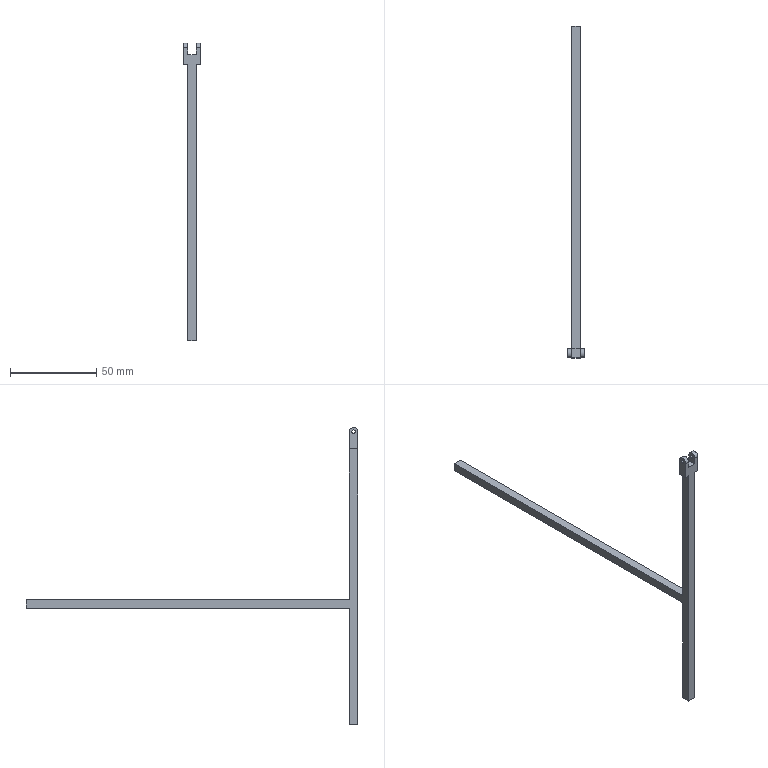Part | SolidWorks | features ICE 4, Extrusion 1 | 1 solid | 22 faces | box 10 x 192.5 x 172.5 mm | volume 9121 mm3 | plane 16 | cylinder 6 | commonest cylinder face diameters 2 x4 5 x2
STEP:
#1=CARTESIAN_POINT('',(2.5,-1.,170.));
#2=VERTEX_POINT('',#1);
#3=CARTESIAN_POINT('',(2.5,1.,170.));
#4=VERTEX_POINT('',#3);
#5=CARTESIAN_POINT('',(2.5,0.,170.));
#6=DIRECTION('',(1.,0.,0.));
#7=DIRECTION('',(0.,1.,0.));
#8=AXIS2_PLACEMENT_3D('',#5,#6,#7);
#9=CIRCLE('',#8,1.);
#10=EDGE_CURVE('',#2,#4,#9,.T.);
#11=ORIENTED_EDGE('',*,*,#10,.F.);
#12=CARTESIAN_POINT('',(5.,-1.,170.));
#13=VERTEX_POINT('',#12);
#14=CARTESIAN_POINT('',(-5.,-1.,170.));
#15=DIRECTION('',(1.,0.,0.));
#16=VECTOR('',#15,1000.);
#17=LINE('',#14,#16);
#18=EDGE_CURVE('',#2,#13,#17,.T.);
#19=ORIENTED_EDGE('',*,*,#18,.T.);
#20=CARTESIAN_POINT('',(5.,1.,170.));
#21=VERTEX_POINT('',#20);
#22=CARTESIAN_POINT('',(5.,0.,170.));
#23=DIRECTION('',(-1.,0.,0.));
#24=DIRECTION('',(0.,-1.,0.));
#25=AXIS2_PLACEMENT_3D('',#22,#23,#24);
#26=CIRCLE('',#25,1.);
#27=EDGE_CURVE('',#21,#13,#26,.T.);
#28=ORIENTED_EDGE('',*,*,#27,.F.);
#29=CARTESIAN_POINT('',(-5.,1.,170.));
#30=DIRECTION('',(1.,0.,0.));
#31=VECTOR('',#30,1000.);
#32=LINE('',#29,#31);
#33=EDGE_CURVE('',#4,#21,#32,.T.);
#34=ORIENTED_EDGE('',*,*,#33,.F.);
#35=EDGE_LOOP('',(#11,#19,#28,#34));
#36=FACE_OUTER_BOUND('',#35,.T.);
#37=CARTESIAN_POINT('',(-5.,0.,170.));
#38=DIRECTION('',(1.,0.,0.));
#39=DIRECTION('',(0.,1.,0.));
#40=AXIS2_PLACEMENT_3D('',#37,#38,#39);
#41=CYLINDRICAL_SURFACE('',#40,1.);
#42=ADVANCED_FACE('',(#36),#41,.F.);
#43=CARTESIAN_POINT('',(-5.,-1.,170.));
#44=VERTEX_POINT('',#43);
#45=CARTESIAN_POINT('',(-5.,1.,170.));
#46=VERTEX_POINT('',#45);
#47=CARTESIAN_POINT('',(-5.,0.,170.));
#48=DIRECTION('',(1.,0.,0.));
#49=DIRECTION('',(0.,1.,0.));
#50=AXIS2_PLACEMENT_3D('',#47,#48,#49);
#51=CIRCLE('',#50,1.);
#52=EDGE_CURVE('',#44,#46,#51,.T.);
#53=ORIENTED_EDGE('',*,*,#52,.F.);
#54=CARTESIAN_POINT('',(-2.5,-1.,170.));
#55=VERTEX_POINT('',#54);
#56=CARTESIAN_POINT('',(-5.,-1.,170.));
#57=DIRECTION('',(1.,0.,0.));
#58=VECTOR('',#57,1000.);
#59=LINE('',#56,#58);
#60=EDGE_CURVE('',#44,#55,#59,.T.);
#61=ORIENTED_EDGE('',*,*,#60,.T.);
#62=CARTESIAN_POINT('',(-2.5,1.,170.));
#63=VERTEX_POINT('',#62);
#64=CARTESIAN_POINT('',(-2.5,0.,170.));
#65=DIRECTION('',(-1.,0.,0.));
#66=DIRECTION('',(0.,-1.,0.));
#67=AXIS2_PLACEMENT_3D('',#64,#65,#66);
#68=CIRCLE('',#67,1.);
#69=EDGE_CURVE('',#63,#55,#68,.T.);
#70=ORIENTED_EDGE('',*,*,#69,.F.);
#71=CARTESIAN_POINT('',(-5.,1.,170.));
#72=DIRECTION('',(1.,0.,0.));
#73=VECTOR('',#72,1000.);
#74=LINE('',#71,#73);
#75=EDGE_CURVE('',#46,#63,#74,.T.);
#76=ORIENTED_EDGE('',*,*,#75,.F.);
#77=EDGE_LOOP('',(#53,#61,#70,#76));
#78=FACE_OUTER_BOUND('',#77,.T.);
#79=CARTESIAN_POINT('',(-5.,0.,170.));
#80=DIRECTION('',(1.,0.,0.));
#81=DIRECTION('',(0.,1.,0.));
#82=AXIS2_PLACEMENT_3D('',#79,#80,#81);
#83=CYLINDRICAL_SURFACE('',#82,1.);
#84=ADVANCED_FACE('',(#78),#83,.F.);
#85=CARTESIAN_POINT('',(2.5,2.5,67.5));
#86=VERTEX_POINT('',#85);
#87=CARTESIAN_POINT('',(-2.5,2.5,67.5));
#88=VERTEX_POINT('',#87);
#89=CARTESIAN_POINT('',(-2.5,2.5,67.5));
#90=DIRECTION('',(-1.,0.,0.));
#91=VECTOR('',#90,1000.);
#92=LINE('',#89,#91);
#93=EDGE_CURVE('',#86,#88,#92,.T.);
#94=ORIENTED_EDGE('',*,*,#93,.F.);
#95=CARTESIAN_POINT('',(2.5,2.5,0.));
#96=VERTEX_POINT('',#95);
#97=CARTESIAN_POINT('',(2.5,2.5,160.));
#98=DIRECTION('',(0.,0.,-1.));
#99=VECTOR('',#98,1000.);
#100=LINE('',#97,#99);
#101=EDGE_CURVE('',#86,#96,#100,.T.);
#102=ORIENTED_EDGE('',*,*,#101,.T.);
#103=CARTESIAN_POINT('',(-2.5,2.5,0.));
#104=VERTEX_POINT('',#103);
#105=CARTESIAN_POINT('',(-2.5,2.5,0.));
#106=DIRECTION('',(-1.,0.,0.));
#107=VECTOR('',#106,1000.);
#108=LINE('',#105,#107);
#109=EDGE_CURVE('',#96,#104,#108,.T.);
#110=ORIENTED_EDGE('',*,*,#109,.T.);
#111=CARTESIAN_POINT('',(-2.5,2.5,160.));
#112=DIRECTION('',(0.,0.,-1.));
#113=VECTOR('',#112,1000.);
#114=LINE('',#111,#113);
#115=EDGE_CURVE('',#88,#104,#114,.T.);
#116=ORIENTED_EDGE('',*,*,#115,.F.);
#117=EDGE_LOOP('',(#94,#102,#110,#116));
#118=FACE_OUTER_BOUND('',#117,.T.);
#119=CARTESIAN_POINT('',(-2.5,2.5,160.));
#120=DIRECTION('',(0.,-1.,0.));
#121=DIRECTION('',(0.,0.,-1.));
#122=AXIS2_PLACEMENT_3D('',#119,#120,#121);
#123=PLANE('',#122);
#124=ADVANCED_FACE('',(#118),#123,.F.);
#125=CARTESIAN_POINT('',(-2.5,2.5,72.5));
#126=VERTEX_POINT('',#125);
#127=CARTESIAN_POINT('',(2.5,2.5,72.5));
#128=VERTEX_POINT('',#127);
#129=CARTESIAN_POINT('',(-2.5,2.5,72.5));
#130=DIRECTION('',(1.,0.,0.));
#131=VECTOR('',#130,1000.);
#132=LINE('',#129,#131);
#133=EDGE_CURVE('',#126,#128,#132,.T.);
#134=ORIENTED_EDGE('',*,*,#133,.F.);
#135=CARTESIAN_POINT('',(-2.5,2.5,160.));
#136=VERTEX_POINT('',#135);
#137=CARTESIAN_POINT('',(-2.5,2.5,160.));
#138=DIRECTION('',(0.,0.,-1.));
#139=VECTOR('',#138,1000.);
#140=LINE('',#137,#139);
#141=EDGE_CURVE('',#136,#126,#140,.T.);
#142=ORIENTED_EDGE('',*,*,#141,.F.);
#143=CARTESIAN_POINT('',(-5.,2.5,160.));
#144=VERTEX_POINT('',#143);
#145=CARTESIAN_POINT('',(-5.,2.5,160.));
#146=DIRECTION('',(-1.,0.,0.));
#147=VECTOR('',#146,1000.);
#148=LINE('',#145,#147);
#149=EDGE_CURVE('',#136,#144,#148,.T.);
#150=ORIENTED_EDGE('',*,*,#149,.T.);
#151=CARTESIAN_POINT('',(-5.,2.5,170.));
#152=VERTEX_POINT('',#151);
#153=CARTESIAN_POINT('',(-5.,2.5,178.));
#154=DIRECTION('',(0.,0.,-1.));
#155=VECTOR('',#154,1000.);
#156=LINE('',#153,#155);
#157=EDGE_CURVE('',#152,#144,#156,.T.);
#158=ORIENTED_EDGE('',*,*,#157,.F.);
#159=CARTESIAN_POINT('',(-2.5,2.5,170.));
#160=VERTEX_POINT('',#159);
#161=CARTESIAN_POINT('',(-5.,2.5,170.));
#162=DIRECTION('',(1.,0.,0.));
#163=VECTOR('',#162,1000.);
#164=LINE('',#161,#163);
#165=EDGE_CURVE('',#152,#160,#164,.T.);
#166=ORIENTED_EDGE('',*,*,#165,.T.);
#167=CARTESIAN_POINT('',(-2.5,2.5,166.));
#168=VERTEX_POINT('',#167);
#169=CARTESIAN_POINT('',(-2.5,2.5,160.));
#170=DIRECTION('',(0.,0.,-1.));
#171=VECTOR('',#170,1000.);
#172=LINE('',#169,#171);
#173=EDGE_CURVE('',#160,#168,#172,.T.);
#174=ORIENTED_EDGE('',*,*,#173,.T.);
#175=CARTESIAN_POINT('',(2.5,2.5,166.));
#176=VERTEX_POINT('',#175);
#177=CARTESIAN_POINT('',(-2.5,2.5,166.));
#178=DIRECTION('',(-1.,0.,0.));
#179=VECTOR('',#178,1000.);
#180=LINE('',#177,#179);
#181=EDGE_CURVE('',#176,#168,#180,.T.);
#182=ORIENTED_EDGE('',*,*,#181,.F.);
#183=CARTESIAN_POINT('',(2.5,2.5,170.));
#184=VERTEX_POINT('',#183);
#185=CARTESIAN_POINT('',(2.5,2.5,160.));
#186=DIRECTION('',(0.,0.,1.));
#187=VECTOR('',#186,1000.);
#188=LINE('',#185,#187);
#189=EDGE_CURVE('',#176,#184,#188,.T.);
#190=ORIENTED_EDGE('',*,*,#189,.T.);
#191=CARTESIAN_POINT('',(5.,2.5,170.));
#192=VERTEX_POINT('',#191);
#193=CARTESIAN_POINT('',(-5.,2.5,170.));
#194=DIRECTION('',(1.,0.,0.));
#195=VECTOR('',#194,1000.);
#196=LINE('',#193,#195);
#197=EDGE_CURVE('',#184,#192,#196,.T.);
#198=ORIENTED_EDGE('',*,*,#197,.T.);
#199=CARTESIAN_POINT('',(5.,2.5,160.));
#200=VERTEX_POINT('',#199);
#201=CARTESIAN_POINT('',(5.,2.5,178.));
#202=DIRECTION('',(0.,0.,-1.));
#203=VECTOR('',#202,1000.);
#204=LINE('',#201,#203);
#205=EDGE_CURVE('',#192,#200,#204,.T.);
#206=ORIENTED_EDGE('',*,*,#205,.T.);
#207=CARTESIAN_POINT('',(2.5,2.5,160.));
#208=VERTEX_POINT('',#207);
#209=CARTESIAN_POINT('',(-5.,2.5,160.));
#210=DIRECTION('',(-1.,0.,0.));
#211=VECTOR('',#210,1000.);
#212=LINE('',#209,#211);
#213=EDGE_CURVE('',#200,#208,#212,.T.);
#214=ORIENTED_EDGE('',*,*,#213,.T.);
#215=CARTESIAN_POINT('',(2.5,2.5,160.));
#216=DIRECTION('',(0.,0.,-1.));
#217=VECTOR('',#216,1000.);
#218=LINE('',#215,#217);
#219=EDGE_CURVE('',#208,#128,#218,.T.);
#220=ORIENTED_EDGE('',*,*,#219,.T.);
#221=EDGE_LOOP('',(#134,#142,#150,#158,#166,#174,#182,#190,#198,#206,#214,#220));
#222=FACE_OUTER_BOUND('',#221,.T.);
#223=CARTESIAN_POINT('',(-2.5,2.5,160.));
#224=DIRECTION('',(0.,-1.,0.));
#225=DIRECTION('',(0.,0.,-1.));
#226=AXIS2_PLACEMENT_3D('',#223,#224,#225);
#227=PLANE('',#226);
#228=ADVANCED_FACE('',(#222),#227,.F.);
#229=ORIENTED_EDGE('',*,*,#101,.F.);
#230=CARTESIAN_POINT('',(2.5,190.,67.5));
#231=VERTEX_POINT('',#230);
#232=CARTESIAN_POINT('',(2.5,190.,67.5));
#233=DIRECTION('',(0.,-1.,0.));
#234=VECTOR('',#233,1000.);
#235=LINE('',#232,#234);
#236=EDGE_CURVE('',#231,#86,#235,.T.);
#237=ORIENTED_EDGE('',*,*,#236,.F.);
#238=CARTESIAN_POINT('',(2.5,190.,72.5));
#239=VERTEX_POINT('',#238);
#240=CARTESIAN_POINT('',(2.5,190.,67.5));
#241=DIRECTION('',(0.,0.,-1.));
#242=VECTOR('',#241,1000.);
#243=LINE('',#240,#242);
#244=EDGE_CURVE('',#239,#231,#243,.T.);
#245=ORIENTED_EDGE('',*,*,#244,.F.);
#246=CARTESIAN_POINT('',(2.5,190.,72.5));
#247=DIRECTION('',(0.,-1.,0.));
#248=VECTOR('',#247,1000.);
#249=LINE('',#246,#248);
#250=EDGE_CURVE('',#239,#128,#249,.T.);
#251=ORIENTED_EDGE('',*,*,#250,.T.);
#252=ORIENTED_EDGE('',*,*,#219,.F.);
#253=CARTESIAN_POINT('',(2.5,-2.5,160.));
#254=VERTEX_POINT('',#253);
#255=CARTESIAN_POINT('',(2.5,2.5,160.));
#256=DIRECTION('',(0.,1.,0.));
#257=VECTOR('',#256,1000.);
#258=LINE('',#255,#257);
#259=EDGE_CURVE('',#254,#208,#258,.T.);
#260=ORIENTED_EDGE('',*,*,#259,.F.);
#261=CARTESIAN_POINT('',(2.5,-2.5,0.));
#262=VERTEX_POINT('',#261);
#263=CARTESIAN_POINT('',(2.5,-2.5,160.));
#264=DIRECTION('',(0.,0.,-1.));
#265=VECTOR('',#264,1000.);
#266=LINE('',#263,#265);
#267=EDGE_CURVE('',#254,#262,#266,.T.);
#268=ORIENTED_EDGE('',*,*,#267,.T.);
#269=CARTESIAN_POINT('',(2.5,2.5,0.));
#270=DIRECTION('',(0.,1.,0.));
#271=VECTOR('',#270,1000.);
#272=LINE('',#269,#271);
#273=EDGE_CURVE('',#262,#96,#272,.T.);
#274=ORIENTED_EDGE('',*,*,#273,.T.);
#275=EDGE_LOOP('',(#229,#237,#245,#251,#252,#260,#268,#274));
#276=FACE_OUTER_BOUND('',#275,.T.);
#277=CARTESIAN_POINT('',(2.5,2.5,160.));
#278=DIRECTION('',(-1.,0.,0.));
#279=DIRECTION('',(0.,-1.,0.));
#280=AXIS2_PLACEMENT_3D('',#277,#278,#279);
#281=PLANE('',#280);
#282=ADVANCED_FACE('',(#276),#281,.F.);
#283=ORIENTED_EDGE('',*,*,#141,.T.);
#284=CARTESIAN_POINT('',(-2.5,190.,72.5));
#285=VERTEX_POINT('',#284);
#286=CARTESIAN_POINT('',(-2.5,190.,72.5));
#287=DIRECTION('',(0.,-1.,0.));
#288=VECTOR('',#287,1000.);
#289=LINE('',#286,#288);
#290=EDGE_CURVE('',#285,#126,#289,.T.);
#291=ORIENTED_EDGE('',*,*,#290,.F.);
#292=CARTESIAN_POINT('',(-2.5,190.,67.5));
#293=VERTEX_POINT('',#292);
#294=CARTESIAN_POINT('',(-2.5,190.,67.5));
#295=DIRECTION('',(0.,0.,1.));
#296=VECTOR('',#295,1000.);
#297=LINE('',#294,#296);
#298=EDGE_CURVE('',#293,#285,#297,.T.);
#299=ORIENTED_EDGE('',*,*,#298,.F.);
#300=CARTESIAN_POINT('',(-2.5,190.,67.5));
#301=DIRECTION('',(0.,-1.,0.));
#302=VECTOR('',#301,1000.);
#303=LINE('',#300,#302);
#304=EDGE_CURVE('',#293,#88,#303,.T.);
#305=ORIENTED_EDGE('',*,*,#304,.T.);
#306=ORIENTED_EDGE('',*,*,#115,.T.);
#307=CARTESIAN_POINT('',(-2.5,-2.5,0.));
#308=VERTEX_POINT('',#307);
#309=CARTESIAN_POINT('',(-2.5,2.5,0.));
#310=DIRECTION('',(0.,-1.,0.));
#311=VECTOR('',#310,1000.);
#312=LINE('',#309,#311);
#313=EDGE_CURVE('',#104,#308,#312,.T.);
#314=ORIENTED_EDGE('',*,*,#313,.T.);
#315=CARTESIAN_POINT('',(-2.5,-2.5,160.));
#316=VERTEX_POINT('',#315);
#317=CARTESIAN_POINT('',(-2.5,-2.5,160.));
#318=DIRECTION('',(0.,0.,-1.));
#319=VECTOR('',#318,1000.);
#320=LINE('',#317,#319);
#321=EDGE_CURVE('',#316,#308,#320,.T.);
#322=ORIENTED_EDGE('',*,*,#321,.F.);
#323=CARTESIAN_POINT('',(-2.5,2.5,160.));
#324=DIRECTION('',(0.,-1.,0.));
#325=VECTOR('',#324,1000.);
#326=LINE('',#323,#325);
#327=EDGE_CURVE('',#136,#316,#326,.T.);
#328=ORIENTED_EDGE('',*,*,#327,.F.);
#329=EDGE_LOOP('',(#283,#291,#299,#305,#306,#314,#322,#328));
#330=FACE_OUTER_BOUND('',#329,.T.);
#331=CARTESIAN_POINT('',(-2.5,2.5,160.));
#332=DIRECTION('',(1.,0.,0.));
#333=DIRECTION('',(0.,1.,0.));
#334=AXIS2_PLACEMENT_3D('',#331,#332,#333);
#335=PLANE('',#334);
#336=ADVANCED_FACE('',(#330),#335,.F.);
#337=CARTESIAN_POINT('',(5.,-2.5,170.));
#338=VERTEX_POINT('',#337);
#339=CARTESIAN_POINT('',(5.,-2.5,160.));
#340=VERTEX_POINT('',#339);
#341=CARTESIAN_POINT('',(5.,-2.5,178.));
#342=DIRECTION('',(0.,0.,-1.));
#343=VECTOR('',#342,1000.);
#344=LINE('',#341,#343);
#345=EDGE_CURVE('',#338,#340,#344,.T.);
#346=ORIENTED_EDGE('',*,*,#345,.F.);
#347=CARTESIAN_POINT('',(2.5,-2.5,170.));
#348=VERTEX_POINT('',#347);
#349=CARTESIAN_POINT('',(-5.,-2.5,170.));
#350=DIRECTION('',(1.,0.,0.));
#351=VECTOR('',#350,1000.);
#352=LINE('',#349,#351);
#353=EDGE_CURVE('',#348,#338,#352,.T.);
#354=ORIENTED_EDGE('',*,*,#353,.F.);
#355=CARTESIAN_POINT('',(2.5,-2.5,166.));
#356=VERTEX_POINT('',#355);
#357=CARTESIAN_POINT('',(2.5,-2.5,160.));
#358=DIRECTION('',(0.,0.,-1.));
#359=VECTOR('',#358,1000.);
#360=LINE('',#357,#359);
#361=EDGE_CURVE('',#348,#356,#360,.T.);
#362=ORIENTED_EDGE('',*,*,#361,.T.);
#363=CARTESIAN_POINT('',(-2.5,-2.5,166.));
#364=VERTEX_POINT('',#363);
#365=CARTESIAN_POINT('',(-2.5,-2.5,166.));
#366=DIRECTION('',(1.,0.,0.));
#367=VECTOR('',#366,1000.);
#368=LINE('',#365,#367);
#369=EDGE_CURVE('',#364,#356,#368,.T.);
#370=ORIENTED_EDGE('',*,*,#369,.F.);
#371=CARTESIAN_POINT('',(-2.5,-2.5,170.));
#372=VERTEX_POINT('',#371);
#373=CARTESIAN_POINT('',(-2.5,-2.5,160.));
#374=DIRECTION('',(0.,0.,1.));
#375=VECTOR('',#374,1000.);
#376=LINE('',#373,#375);
#377=EDGE_CURVE('',#364,#372,#376,.T.);
#378=ORIENTED_EDGE('',*,*,#377,.T.);
#379=CARTESIAN_POINT('',(-5.,-2.5,170.));
#380=VERTEX_POINT('',#379);
#381=CARTESIAN_POINT('',(-5.,-2.5,170.));
#382=DIRECTION('',(1.,0.,0.));
#383=VECTOR('',#382,1000.);
#384=LINE('',#381,#383);
#385=EDGE_CURVE('',#380,#372,#384,.T.);
#386=ORIENTED_EDGE('',*,*,#385,.F.);
#387=CARTESIAN_POINT('',(-5.,-2.5,160.));
#388=VERTEX_POINT('',#387);
#389=CARTESIAN_POINT('',(-5.,-2.5,178.));
#390=DIRECTION('',(0.,0.,-1.));
#391=VECTOR('',#390,1000.);
#392=LINE('',#389,#391);
#393=EDGE_CURVE('',#380,#388,#392,.T.);
#394=ORIENTED_EDGE('',*,*,#393,.T.);
#395=CARTESIAN_POINT('',(-5.,-2.5,160.));
#396=DIRECTION('',(1.,0.,0.));
#397=VECTOR('',#396,1000.);
#398=LINE('',#395,#397);
#399=EDGE_CURVE('',#388,#316,#398,.T.);
#400=ORIENTED_EDGE('',*,*,#399,.T.);
#401=ORIENTED_EDGE('',*,*,#321,.T.);
#402=CARTESIAN_POINT('',(-2.5,-2.5,0.));
#403=DIRECTION('',(1.,0.,0.));
#404=VECTOR('',#403,1000.);
#405=LINE('',#402,#404);
#406=EDGE_CURVE('',#308,#262,#405,.T.);
#407=ORIENTED_EDGE('',*,*,#406,.T.);
#408=ORIENTED_EDGE('',*,*,#267,.F.);
#409=CARTESIAN_POINT('',(-5.,-2.5,160.));
#410=DIRECTION('',(1.,0.,0.));
#411=VECTOR('',#410,1000.);
#412=LINE('',#409,#411);
#413=EDGE_CURVE('',#254,#340,#412,.T.);
#414=ORIENTED_EDGE('',*,*,#413,.T.);
#415=EDGE_LOOP('',(#346,#354,#362,#370,#378,#386,#394,#400,#401,#407,#408,#414));
#416=FACE_OUTER_BOUND('',#415,.T.);
#417=CARTESIAN_POINT('',(-2.5,-2.5,160.));
#418=DIRECTION('',(0.,1.,0.));
#419=DIRECTION('',(0.,0.,1.));
#420=AXIS2_PLACEMENT_3D('',#417,#418,#419);
#421=PLANE('',#420);
#422=ADVANCED_FACE('',(#416),#421,.F.);
#423=ORIENTED_EDGE('',*,*,#273,.F.);
#424=ORIENTED_EDGE('',*,*,#406,.F.);
#425=ORIENTED_EDGE('',*,*,#313,.F.);
#426=ORIENTED_EDGE('',*,*,#109,.F.);
#427=EDGE_LOOP('',(#423,#424,#425,#426));
#428=FACE_OUTER_BOUND('',#427,.T.);
#429=CARTESIAN_POINT('',(0.,0.,0.));
#430=DIRECTION('',(0.,0.,1.));
#431=DIRECTION('',(1.,0.,0.));
#432=AXIS2_PLACEMENT_3D('',#429,#430,#431);
#433=PLANE('',#432);
#434=ADVANCED_FACE('',(#428),#433,.F.);
#435=ORIENTED_EDGE('',*,*,#413,.F.);
#436=ORIENTED_EDGE('',*,*,#259,.T.);
#437=ORIENTED_EDGE('',*,*,#213,.F.);
#438=CARTESIAN_POINT('',(5.,2.5,160.));
#439=DIRECTION('',(0.,1.,0.));
#440=VECTOR('',#439,1000.);
#441=LINE('',#438,#440);
#442=EDGE_CURVE('',#340,#200,#441,.T.);
#443=ORIENTED_EDGE('',*,*,#442,.F.);
#444=EDGE_LOOP('',(#435,#436,#437,#443));
#445=FACE_OUTER_BOUND('',#444,.T.);
#446=CARTESIAN_POINT('',(0.,0.,160.));
#447=DIRECTION('',(0.,0.,1.));
#448=DIRECTION('',(1.,0.,0.));
#449=AXIS2_PLACEMENT_3D('',#446,#447,#448);
#450=PLANE('',#449);
#451=ADVANCED_FACE('',(#445),#450,.F.);
#452=ORIENTED_EDGE('',*,*,#149,.F.);
#453=ORIENTED_EDGE('',*,*,#327,.T.);
#454=ORIENTED_EDGE('',*,*,#399,.F.);
#455=CARTESIAN_POINT('',(-5.,2.5,160.));
#456=DIRECTION('',(0.,-1.,0.));
#457=VECTOR('',#456,1000.);
#458=LINE('',#455,#457);
#459=EDGE_CURVE('',#144,#388,#458,.T.);
#460=ORIENTED_EDGE('',*,*,#459,.F.);
#461=EDGE_LOOP('',(#452,#453,#454,#460));
#462=FACE_OUTER_BOUND('',#461,.T.);
#463=CARTESIAN_POINT('',(0.,0.,160.));
#464=DIRECTION('',(0.,0.,1.));
#465=DIRECTION('',(1.,0.,0.));
#466=AXIS2_PLACEMENT_3D('',#463,#464,#465);
#467=PLANE('',#466);
#468=ADVANCED_FACE('',(#462),#467,.F.);
#469=ORIENTED_EDGE('',*,*,#27,.T.);
#470=CARTESIAN_POINT('',(5.,0.,170.));
#471=DIRECTION('',(-1.,0.,0.));
#472=DIRECTION('',(0.,-1.,0.));
#473=AXIS2_PLACEMENT_3D('',#470,#471,#472);
#474=CIRCLE('',#473,1.);
#475=EDGE_CURVE('',#13,#21,#474,.T.);
#476=ORIENTED_EDGE('',*,*,#475,.T.);
#477=EDGE_LOOP('',(#469,#476));
#478=FACE_BOUND('',#477,.T.);
#479=ORIENTED_EDGE('',*,*,#205,.F.);
#480=CARTESIAN_POINT('',(5.,0.,170.));
#481=DIRECTION('',(-1.,0.,0.));
#482=DIRECTION('',(0.,1.,0.));
#483=AXIS2_PLACEMENT_3D('',#480,#481,#482);
#484=CIRCLE('',#483,2.5);
#485=EDGE_CURVE('',#338,#192,#484,.T.);
#486=ORIENTED_EDGE('',*,*,#485,.F.);
#487=ORIENTED_EDGE('',*,*,#345,.T.);
#488=ORIENTED_EDGE('',*,*,#442,.T.);
#489=EDGE_LOOP('',(#479,#486,#487,#488));
#490=FACE_OUTER_BOUND('',#489,.T.);
#491=CARTESIAN_POINT('',(5.,2.5,178.));
#492=DIRECTION('',(-1.,0.,0.));
#493=DIRECTION('',(0.,-1.,0.));
#494=AXIS2_PLACEMENT_3D('',#491,#492,#493);
#495=PLANE('',#494);
#496=ADVANCED_FACE('',(#478,#490),#495,.F.);
#497=CARTESIAN_POINT('',(-5.,0.,170.));
#498=DIRECTION('',(1.,0.,0.));
#499=DIRECTION('',(0.,1.,0.));
#500=AXIS2_PLACEMENT_3D('',#497,#498,#499);
#501=CIRCLE('',#500,1.);
#502=EDGE_CURVE('',#46,#44,#501,.T.);
#503=ORIENTED_EDGE('',*,*,#502,.T.);
#504=ORIENTED_EDGE('',*,*,#52,.T.);
#505=EDGE_LOOP('',(#503,#504));
#506=FACE_BOUND('',#505,.T.);
#507=ORIENTED_EDGE('',*,*,#393,.F.);
#508=CARTESIAN_POINT('',(-5.,0.,170.));
#509=DIRECTION('',(-1.,0.,0.));
#510=DIRECTION('',(0.,1.,0.));
#511=AXIS2_PLACEMENT_3D('',#508,#509,#510);
#512=CIRCLE('',#511,2.5);
#513=EDGE_CURVE('',#380,#152,#512,.T.);
#514=ORIENTED_EDGE('',*,*,#513,.T.);
#515=ORIENTED_EDGE('',*,*,#157,.T.);
#516=ORIENTED_EDGE('',*,*,#459,.T.);
#517=EDGE_LOOP('',(#507,#514,#515,#516));
#518=FACE_OUTER_BOUND('',#517,.T.);
#519=CARTESIAN_POINT('',(-5.,2.5,178.));
#520=DIRECTION('',(1.,0.,0.));
#521=DIRECTION('',(0.,0.,-1.));
#522=AXIS2_PLACEMENT_3D('',#519,#520,#521);
#523=PLANE('',#522);
#524=ADVANCED_FACE('',(#506,#518),#523,.F.);
#525=ORIENTED_EDGE('',*,*,#181,.T.);
#526=CARTESIAN_POINT('',(-2.5,9.679,166.));
#527=DIRECTION('',(0.,-1.,0.));
#528=VECTOR('',#527,1000.);
#529=LINE('',#526,#528);
#530=EDGE_CURVE('',#168,#364,#529,.T.);
#531=ORIENTED_EDGE('',*,*,#530,.T.);
#532=ORIENTED_EDGE('',*,*,#369,.T.);
#533=CARTESIAN_POINT('',(2.5,9.679,166.));
#534=DIRECTION('',(0.,1.,0.));
#535=VECTOR('',#534,1000.);
#536=LINE('',#533,#535);
#537=EDGE_CURVE('',#356,#176,#536,.T.);
#538=ORIENTED_EDGE('',*,*,#537,.T.);
#539=EDGE_LOOP('',(#525,#531,#532,#538));
#540=FACE_OUTER_BOUND('',#539,.T.);
#541=CARTESIAN_POINT('',(0.,0.,166.));
#542=DIRECTION('',(0.,0.,1.));
#543=DIRECTION('',(1.,0.,0.));
#544=AXIS2_PLACEMENT_3D('',#541,#542,#543);
#545=PLANE('',#544);
#546=ADVANCED_FACE('',(#540),#545,.T.);
#547=CARTESIAN_POINT('',(2.5,0.,170.));
#548=DIRECTION('',(1.,0.,0.));
#549=DIRECTION('',(0.,1.,0.));
#550=AXIS2_PLACEMENT_3D('',#547,#548,#549);
#551=CIRCLE('',#550,1.);
#552=EDGE_CURVE('',#4,#2,#551,.T.);
#553=ORIENTED_EDGE('',*,*,#552,.T.);
#554=ORIENTED_EDGE('',*,*,#10,.T.);
#555=EDGE_LOOP('',(#553,#554));
#556=FACE_BOUND('',#555,.T.);
#557=ORIENTED_EDGE('',*,*,#361,.F.);
#558=CARTESIAN_POINT('',(2.5,0.,170.));
#559=DIRECTION('',(-1.,0.,0.));
#560=DIRECTION('',(0.,1.,0.));
#561=AXIS2_PLACEMENT_3D('',#558,#559,#560);
#562=CIRCLE('',#561,2.5);
#563=EDGE_CURVE('',#348,#184,#562,.T.);
#564=ORIENTED_EDGE('',*,*,#563,.T.);
#565=ORIENTED_EDGE('',*,*,#189,.F.);
#566=ORIENTED_EDGE('',*,*,#537,.F.);
#567=EDGE_LOOP('',(#557,#564,#565,#566));
#568=FACE_OUTER_BOUND('',#567,.T.);
#569=CARTESIAN_POINT('',(2.5,9.679,166.));
#570=DIRECTION('',(1.,0.,0.));
#571=DIRECTION('',(0.,1.,0.));
#572=AXIS2_PLACEMENT_3D('',#569,#570,#571);
#573=PLANE('',#572);
#574=ADVANCED_FACE('',(#556,#568),#573,.F.);
#575=ORIENTED_EDGE('',*,*,#69,.T.);
#576=CARTESIAN_POINT('',(-2.5,0.,170.));
#577=DIRECTION('',(-1.,0.,0.));
#578=DIRECTION('',(0.,-1.,0.));
#579=AXIS2_PLACEMENT_3D('',#576,#577,#578);
#580=CIRCLE('',#579,1.);
#581=EDGE_CURVE('',#55,#63,#580,.T.);
#582=ORIENTED_EDGE('',*,*,#581,.T.);
#583=EDGE_LOOP('',(#575,#582));
#584=FACE_BOUND('',#583,.T.);
#585=ORIENTED_EDGE('',*,*,#173,.F.);
#586=CARTESIAN_POINT('',(-2.5,0.,170.));
#587=DIRECTION('',(1.,0.,0.));
#588=DIRECTION('',(0.,-1.,0.));
#589=AXIS2_PLACEMENT_3D('',#586,#587,#588);
#590=CIRCLE('',#589,2.5);
#591=EDGE_CURVE('',#160,#372,#590,.T.);
#592=ORIENTED_EDGE('',*,*,#591,.T.);
#593=ORIENTED_EDGE('',*,*,#377,.F.);
#594=ORIENTED_EDGE('',*,*,#530,.F.);
#595=EDGE_LOOP('',(#585,#592,#593,#594));
#596=FACE_OUTER_BOUND('',#595,.T.);
#597=CARTESIAN_POINT('',(-2.5,9.679,166.));
#598=DIRECTION('',(-1.,0.,0.));
#599=DIRECTION('',(0.,-1.,0.));
#600=AXIS2_PLACEMENT_3D('',#597,#598,#599);
#601=PLANE('',#600);
#602=ADVANCED_FACE('',(#584,#596),#601,.F.);
#603=ORIENTED_EDGE('',*,*,#60,.F.);
#604=ORIENTED_EDGE('',*,*,#502,.F.);
#605=ORIENTED_EDGE('',*,*,#75,.T.);
#606=ORIENTED_EDGE('',*,*,#581,.F.);
#607=EDGE_LOOP('',(#603,#604,#605,#606));
#608=FACE_OUTER_BOUND('',#607,.T.);
#609=CARTESIAN_POINT('',(-5.,0.,170.));
#610=DIRECTION('',(1.,0.,0.));
#611=DIRECTION('',(0.,1.,0.));
#612=AXIS2_PLACEMENT_3D('',#609,#610,#611);
#613=CYLINDRICAL_SURFACE('',#612,1.);
#614=ADVANCED_FACE('',(#608),#613,.F.);
#615=ORIENTED_EDGE('',*,*,#165,.F.);
#616=ORIENTED_EDGE('',*,*,#513,.F.);
#617=ORIENTED_EDGE('',*,*,#385,.T.);
#618=ORIENTED_EDGE('',*,*,#591,.F.);
#619=EDGE_LOOP('',(#615,#616,#617,#618));
#620=FACE_OUTER_BOUND('',#619,.T.);
#621=CARTESIAN_POINT('',(-5.,0.,170.));
#622=DIRECTION('',(1.,0.,0.));
#623=DIRECTION('',(0.,1.,0.));
#624=AXIS2_PLACEMENT_3D('',#621,#622,#623);
#625=CYLINDRICAL_SURFACE('',#624,2.5);
#626=ADVANCED_FACE('',(#620),#625,.T.);
#627=ORIENTED_EDGE('',*,*,#18,.F.);
#628=ORIENTED_EDGE('',*,*,#552,.F.);
#629=ORIENTED_EDGE('',*,*,#33,.T.);
#630=ORIENTED_EDGE('',*,*,#475,.F.);
#631=EDGE_LOOP('',(#627,#628,#629,#630));
#632=FACE_OUTER_BOUND('',#631,.T.);
#633=CARTESIAN_POINT('',(-5.,0.,170.));
#634=DIRECTION('',(1.,0.,0.));
#635=DIRECTION('',(0.,1.,0.));
#636=AXIS2_PLACEMENT_3D('',#633,#634,#635);
#637=CYLINDRICAL_SURFACE('',#636,1.);
#638=ADVANCED_FACE('',(#632),#637,.F.);
#639=ORIENTED_EDGE('',*,*,#197,.F.);
#640=ORIENTED_EDGE('',*,*,#563,.F.);
#641=ORIENTED_EDGE('',*,*,#353,.T.);
#642=ORIENTED_EDGE('',*,*,#485,.T.);
#643=EDGE_LOOP('',(#639,#640,#641,#642));
#644=FACE_OUTER_BOUND('',#643,.T.);
#645=CARTESIAN_POINT('',(-5.,0.,170.));
#646=DIRECTION('',(1.,0.,0.));
#647=DIRECTION('',(0.,1.,0.));
#648=AXIS2_PLACEMENT_3D('',#645,#646,#647);
#649=CYLINDRICAL_SURFACE('',#648,2.5);
#650=ADVANCED_FACE('',(#644),#649,.T.);
#651=ORIENTED_EDGE('',*,*,#236,.T.);
#652=ORIENTED_EDGE('',*,*,#93,.T.);
#653=ORIENTED_EDGE('',*,*,#304,.F.);
#654=CARTESIAN_POINT('',(-2.5,190.,67.5));
#655=DIRECTION('',(-1.,0.,0.));
#656=VECTOR('',#655,1000.);
#657=LINE('',#654,#656);
#658=EDGE_CURVE('',#231,#293,#657,.T.);
#659=ORIENTED_EDGE('',*,*,#658,.F.);
#660=EDGE_LOOP('',(#651,#652,#653,#659));
#661=FACE_OUTER_BOUND('',#660,.T.);
#662=CARTESIAN_POINT('',(-2.5,190.,67.5));
#663=DIRECTION('',(0.,0.,1.));
#664=DIRECTION('',(1.,0.,0.));
#665=AXIS2_PLACEMENT_3D('',#662,#663,#664);
#666=PLANE('',#665);
#667=ADVANCED_FACE('',(#661),#666,.F.);
#668=ORIENTED_EDGE('',*,*,#290,.T.);
#669=ORIENTED_EDGE('',*,*,#133,.T.);
#670=ORIENTED_EDGE('',*,*,#250,.F.);
#671=CARTESIAN_POINT('',(-2.5,190.,72.5));
#672=DIRECTION('',(1.,0.,0.));
#673=VECTOR('',#672,1000.);
#674=LINE('',#671,#673);
#675=EDGE_CURVE('',#285,#239,#674,.T.);
#676=ORIENTED_EDGE('',*,*,#675,.F.);
#677=EDGE_LOOP('',(#668,#669,#670,#676));
#678=FACE_OUTER_BOUND('',#677,.T.);
#679=CARTESIAN_POINT('',(-2.5,190.,72.5));
#680=DIRECTION('',(0.,0.,-1.));
#681=DIRECTION('',(-1.,0.,0.));
#682=AXIS2_PLACEMENT_3D('',#679,#680,#681);
#683=PLANE('',#682);
#684=ADVANCED_FACE('',(#678),#683,.F.);
#685=ORIENTED_EDGE('',*,*,#244,.T.);
#686=ORIENTED_EDGE('',*,*,#658,.T.);
#687=ORIENTED_EDGE('',*,*,#298,.T.);
#688=ORIENTED_EDGE('',*,*,#675,.T.);
#689=EDGE_LOOP('',(#685,#686,#687,#688));
#690=FACE_OUTER_BOUND('',#689,.T.);
#691=CARTESIAN_POINT('',(0.,190.,0.));
#692=DIRECTION('',(0.,1.,0.));
#693=DIRECTION('',(0.,0.,1.));
#694=AXIS2_PLACEMENT_3D('',#691,#692,#693);
#695=PLANE('',#694);
#696=ADVANCED_FACE('',(#690),#695,.T.);
#697=CLOSED_SHELL('',(#42,#84,#124,#228,#282,#336,#422,#434,#451,#468,#496,#524,#546,#574,#602,#614,#626,#638,#650,#667,#684,#696));
#698=MANIFOLD_SOLID_BREP('',#697);
#699=CARTESIAN_POINT('',(0.,0.,0.));
#700=DIRECTION('',(0.,0.,1.));
#701=DIRECTION('',(1.,0.,0.));
#702=AXIS2_PLACEMENT_3D('',#699,#700,#701);
#703=(LENGTH_UNIT()NAMED_UNIT(*)SI_UNIT(.MILLI.,.METRE.));
#704=UNCERTAINTY_MEASURE_WITH_UNIT(LENGTH_MEASURE(0.00001),#703,'','');
#705=(NAMED_UNIT(*)PLANE_ANGLE_UNIT()SI_UNIT($,.RADIAN.));
#706=(NAMED_UNIT(*)SI_UNIT($,.STERADIAN.)SOLID_ANGLE_UNIT());
#707=(GEOMETRIC_REPRESENTATION_CONTEXT(3)GLOBAL_UNCERTAINTY_ASSIGNED_CONTEXT((#704))GLOBAL_UNIT_ASSIGNED_CONTEXT((#703,#705,#706))REPRESENTATION_CONTEXT('',''));
#708=ADVANCED_BREP_SHAPE_REPRESENTATION('',(#698,#702),#707);